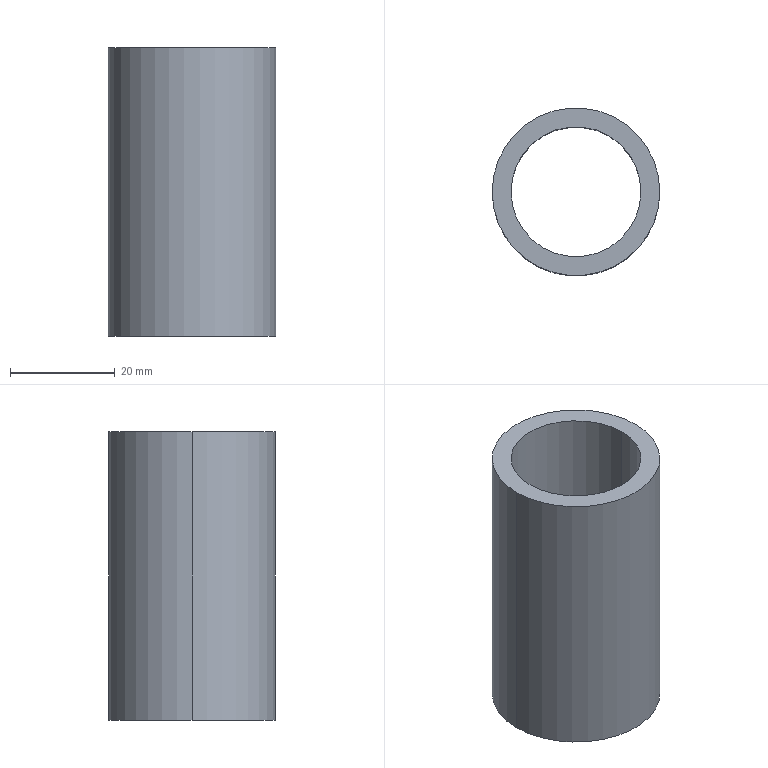Part | SolidWorks | features Extrusion 1 | 1 solid | 6 faces | box 32 x 32 x 55 mm | volume 17666 mm3 | cylinder 4 | plane 2 | commonest cylinder face diameters 24.8 x2 32 x2
STEP:
#1=CARTESIAN_POINT('',(-12.4,0.,27.5));
#2=VERTEX_POINT('',#1);
#3=CARTESIAN_POINT('',(12.4,0.,27.5));
#4=VERTEX_POINT('',#3);
#5=CARTESIAN_POINT('',(0.,0.,27.5));
#6=DIRECTION('',(0.,0.,1.));
#7=DIRECTION('',(1.,0.,0.));
#8=AXIS2_PLACEMENT_3D('',#5,#6,#7);
#9=CIRCLE('',#8,12.4);
#10=EDGE_CURVE('',#2,#4,#9,.T.);
#11=ORIENTED_EDGE('',*,*,#10,.T.);
#12=CARTESIAN_POINT('',(12.4,0.,-27.5));
#13=VERTEX_POINT('',#12);
#14=CARTESIAN_POINT('',(12.4,0.,27.5));
#15=DIRECTION('',(0.,0.,-1.));
#16=VECTOR('',#15,1000.);
#17=LINE('',#14,#16);
#18=EDGE_CURVE('',#4,#13,#17,.T.);
#19=ORIENTED_EDGE('',*,*,#18,.T.);
#20=CARTESIAN_POINT('',(-12.4,0.,-27.5));
#21=VERTEX_POINT('',#20);
#22=CARTESIAN_POINT('',(0.,0.,-27.5));
#23=DIRECTION('',(0.,0.,1.));
#24=DIRECTION('',(1.,0.,0.));
#25=AXIS2_PLACEMENT_3D('',#22,#23,#24);
#26=CIRCLE('',#25,12.4);
#27=EDGE_CURVE('',#21,#13,#26,.T.);
#28=ORIENTED_EDGE('',*,*,#27,.F.);
#29=CARTESIAN_POINT('',(-12.4,0.,27.5));
#30=DIRECTION('',(0.,0.,-1.));
#31=VECTOR('',#30,1000.);
#32=LINE('',#29,#31);
#33=EDGE_CURVE('',#2,#21,#32,.T.);
#34=ORIENTED_EDGE('',*,*,#33,.F.);
#35=EDGE_LOOP('',(#11,#19,#28,#34));
#36=FACE_OUTER_BOUND('',#35,.T.);
#37=CARTESIAN_POINT('',(0.,0.,27.5));
#38=DIRECTION('',(0.,0.,-1.));
#39=DIRECTION('',(-1.,0.,0.));
#40=AXIS2_PLACEMENT_3D('',#37,#38,#39);
#41=CYLINDRICAL_SURFACE('',#40,12.4);
#42=ADVANCED_FACE('',(#36),#41,.F.);
#43=CARTESIAN_POINT('',(16.,0.,27.5));
#44=VERTEX_POINT('',#43);
#45=CARTESIAN_POINT('',(-16.,0.,27.5));
#46=VERTEX_POINT('',#45);
#47=CARTESIAN_POINT('',(0.,0.,27.5));
#48=DIRECTION('',(0.,0.,1.));
#49=DIRECTION('',(1.,0.,0.));
#50=AXIS2_PLACEMENT_3D('',#47,#48,#49);
#51=CIRCLE('',#50,16.);
#52=EDGE_CURVE('',#44,#46,#51,.T.);
#53=ORIENTED_EDGE('',*,*,#52,.F.);
#54=CARTESIAN_POINT('',(16.,0.,-27.5));
#55=VERTEX_POINT('',#54);
#56=CARTESIAN_POINT('',(16.,0.,27.5));
#57=DIRECTION('',(0.,0.,-1.));
#58=VECTOR('',#57,1000.);
#59=LINE('',#56,#58);
#60=EDGE_CURVE('',#44,#55,#59,.T.);
#61=ORIENTED_EDGE('',*,*,#60,.T.);
#62=CARTESIAN_POINT('',(-16.,0.,-27.5));
#63=VERTEX_POINT('',#62);
#64=CARTESIAN_POINT('',(0.,0.,-27.5));
#65=DIRECTION('',(0.,0.,1.));
#66=DIRECTION('',(1.,0.,0.));
#67=AXIS2_PLACEMENT_3D('',#64,#65,#66);
#68=CIRCLE('',#67,16.);
#69=EDGE_CURVE('',#55,#63,#68,.T.);
#70=ORIENTED_EDGE('',*,*,#69,.T.);
#71=CARTESIAN_POINT('',(-16.,0.,27.5));
#72=DIRECTION('',(0.,0.,-1.));
#73=VECTOR('',#72,1000.);
#74=LINE('',#71,#73);
#75=EDGE_CURVE('',#46,#63,#74,.T.);
#76=ORIENTED_EDGE('',*,*,#75,.F.);
#77=EDGE_LOOP('',(#53,#61,#70,#76));
#78=FACE_OUTER_BOUND('',#77,.T.);
#79=CARTESIAN_POINT('',(0.,0.,27.5));
#80=DIRECTION('',(0.,0.,-1.));
#81=DIRECTION('',(-1.,0.,0.));
#82=AXIS2_PLACEMENT_3D('',#79,#80,#81);
#83=CYLINDRICAL_SURFACE('',#82,16.);
#84=ADVANCED_FACE('',(#78),#83,.T.);
#85=CARTESIAN_POINT('',(0.,0.,27.5));
#86=DIRECTION('',(0.,0.,1.));
#87=DIRECTION('',(1.,0.,0.));
#88=AXIS2_PLACEMENT_3D('',#85,#86,#87);
#89=CIRCLE('',#88,16.);
#90=EDGE_CURVE('',#46,#44,#89,.T.);
#91=ORIENTED_EDGE('',*,*,#90,.T.);
#92=ORIENTED_EDGE('',*,*,#52,.T.);
#93=EDGE_LOOP('',(#91,#92));
#94=FACE_OUTER_BOUND('',#93,.T.);
#95=ORIENTED_EDGE('',*,*,#10,.F.);
#96=CARTESIAN_POINT('',(0.,0.,27.5));
#97=DIRECTION('',(0.,0.,1.));
#98=DIRECTION('',(1.,0.,0.));
#99=AXIS2_PLACEMENT_3D('',#96,#97,#98);
#100=CIRCLE('',#99,12.4);
#101=EDGE_CURVE('',#4,#2,#100,.T.);
#102=ORIENTED_EDGE('',*,*,#101,.F.);
#103=EDGE_LOOP('',(#95,#102));
#104=FACE_BOUND('',#103,.T.);
#105=CARTESIAN_POINT('',(0.,0.,27.5));
#106=DIRECTION('',(0.,0.,1.));
#107=DIRECTION('',(1.,0.,0.));
#108=AXIS2_PLACEMENT_3D('',#105,#106,#107);
#109=PLANE('',#108);
#110=ADVANCED_FACE('',(#94,#104),#109,.T.);
#111=CARTESIAN_POINT('',(0.,0.,-27.5));
#112=DIRECTION('',(0.,0.,1.));
#113=DIRECTION('',(1.,0.,0.));
#114=AXIS2_PLACEMENT_3D('',#111,#112,#113);
#115=CIRCLE('',#114,16.);
#116=EDGE_CURVE('',#63,#55,#115,.T.);
#117=ORIENTED_EDGE('',*,*,#116,.F.);
#118=ORIENTED_EDGE('',*,*,#69,.F.);
#119=EDGE_LOOP('',(#117,#118));
#120=FACE_OUTER_BOUND('',#119,.T.);
#121=ORIENTED_EDGE('',*,*,#27,.T.);
#122=CARTESIAN_POINT('',(0.,0.,-27.5));
#123=DIRECTION('',(0.,0.,1.));
#124=DIRECTION('',(1.,0.,0.));
#125=AXIS2_PLACEMENT_3D('',#122,#123,#124);
#126=CIRCLE('',#125,12.4);
#127=EDGE_CURVE('',#13,#21,#126,.T.);
#128=ORIENTED_EDGE('',*,*,#127,.T.);
#129=EDGE_LOOP('',(#121,#128));
#130=FACE_BOUND('',#129,.T.);
#131=CARTESIAN_POINT('',(0.,0.,-27.5));
#132=DIRECTION('',(0.,0.,1.));
#133=DIRECTION('',(1.,0.,0.));
#134=AXIS2_PLACEMENT_3D('',#131,#132,#133);
#135=PLANE('',#134);
#136=ADVANCED_FACE('',(#120,#130),#135,.F.);
#137=ORIENTED_EDGE('',*,*,#60,.F.);
#138=ORIENTED_EDGE('',*,*,#90,.F.);
#139=ORIENTED_EDGE('',*,*,#75,.T.);
#140=ORIENTED_EDGE('',*,*,#116,.T.);
#141=EDGE_LOOP('',(#137,#138,#139,#140));
#142=FACE_OUTER_BOUND('',#141,.T.);
#143=CARTESIAN_POINT('',(0.,0.,27.5));
#144=DIRECTION('',(0.,0.,-1.));
#145=DIRECTION('',(-1.,0.,0.));
#146=AXIS2_PLACEMENT_3D('',#143,#144,#145);
#147=CYLINDRICAL_SURFACE('',#146,16.);
#148=ADVANCED_FACE('',(#142),#147,.T.);
#149=ORIENTED_EDGE('',*,*,#18,.F.);
#150=ORIENTED_EDGE('',*,*,#101,.T.);
#151=ORIENTED_EDGE('',*,*,#33,.T.);
#152=ORIENTED_EDGE('',*,*,#127,.F.);
#153=EDGE_LOOP('',(#149,#150,#151,#152));
#154=FACE_OUTER_BOUND('',#153,.T.);
#155=CARTESIAN_POINT('',(0.,0.,27.5));
#156=DIRECTION('',(0.,0.,-1.));
#157=DIRECTION('',(-1.,0.,0.));
#158=AXIS2_PLACEMENT_3D('',#155,#156,#157);
#159=CYLINDRICAL_SURFACE('',#158,12.4);
#160=ADVANCED_FACE('',(#154),#159,.F.);
#161=CLOSED_SHELL('',(#42,#84,#110,#136,#148,#160));
#162=MANIFOLD_SOLID_BREP('',#161);
#163=CARTESIAN_POINT('',(0.,0.,0.));
#164=DIRECTION('',(0.,0.,1.));
#165=DIRECTION('',(1.,0.,0.));
#166=AXIS2_PLACEMENT_3D('',#163,#164,#165);
#167=(LENGTH_UNIT()NAMED_UNIT(*)SI_UNIT(.MILLI.,.METRE.));
#168=UNCERTAINTY_MEASURE_WITH_UNIT(LENGTH_MEASURE(0.00001),#167,'','');
#169=(NAMED_UNIT(*)PLANE_ANGLE_UNIT()SI_UNIT($,.RADIAN.));
#170=(NAMED_UNIT(*)SI_UNIT($,.STERADIAN.)SOLID_ANGLE_UNIT());
#171=(GEOMETRIC_REPRESENTATION_CONTEXT(3)GLOBAL_UNCERTAINTY_ASSIGNED_CONTEXT((#168))GLOBAL_UNIT_ASSIGNED_CONTEXT((#167,#169,#170))REPRESENTATION_CONTEXT('',''));
#172=ADVANCED_BREP_SHAPE_REPRESENTATION('',(#162,#166),#171);